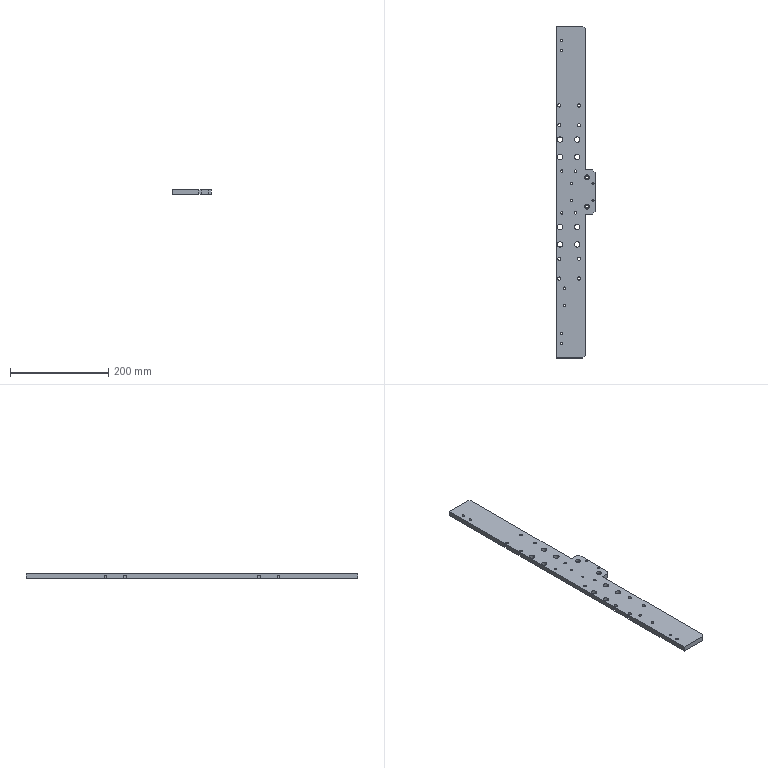Part | SolidWorks | features HoleWzd 7, Chamfer 1, Cut 1, Extrusion 1, ICE 1 | 1 solid | 104 faces | box 78 x 675 x 10 mm | volume 392001 mm3 | cylinder 80 | plane 24 | commonest cylinder face diameters 11 x28 5 x20 6.6 x16 4.2 x8 5.5 x4 10 x4